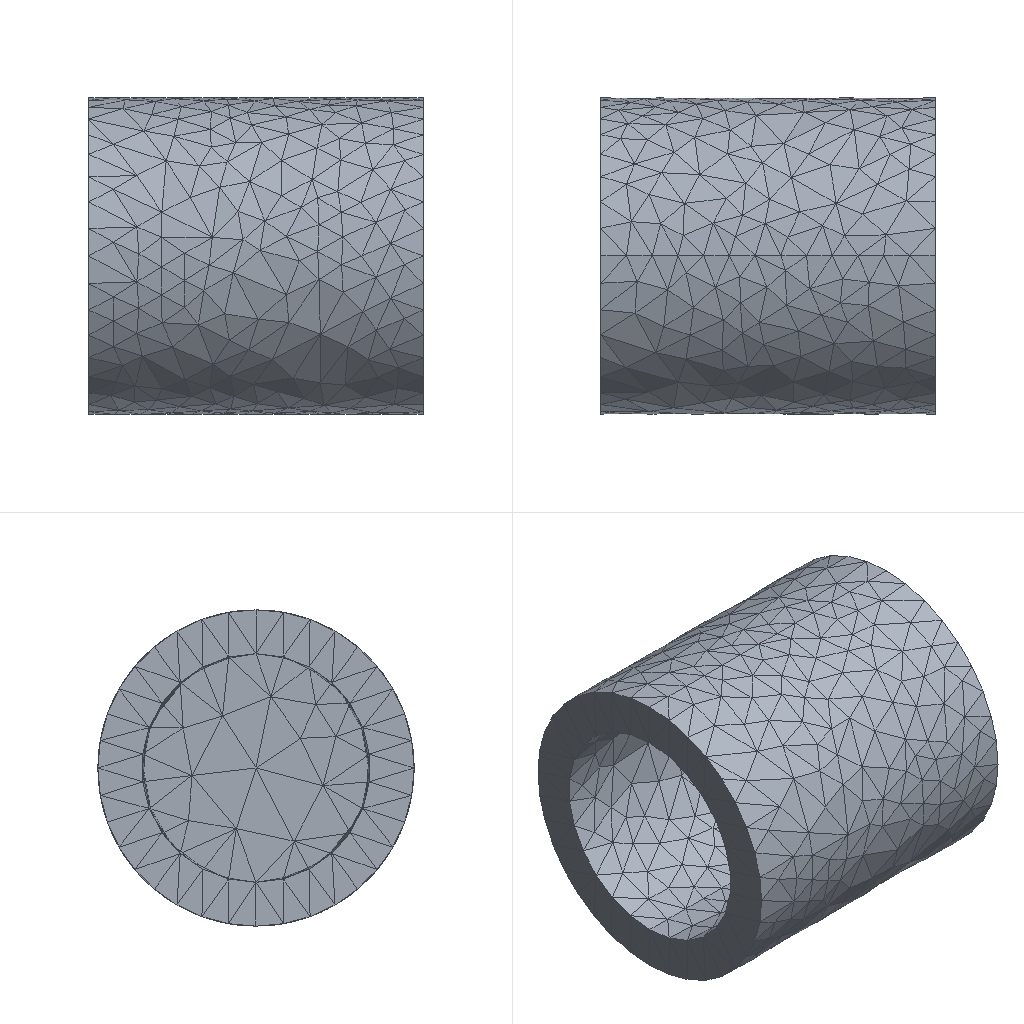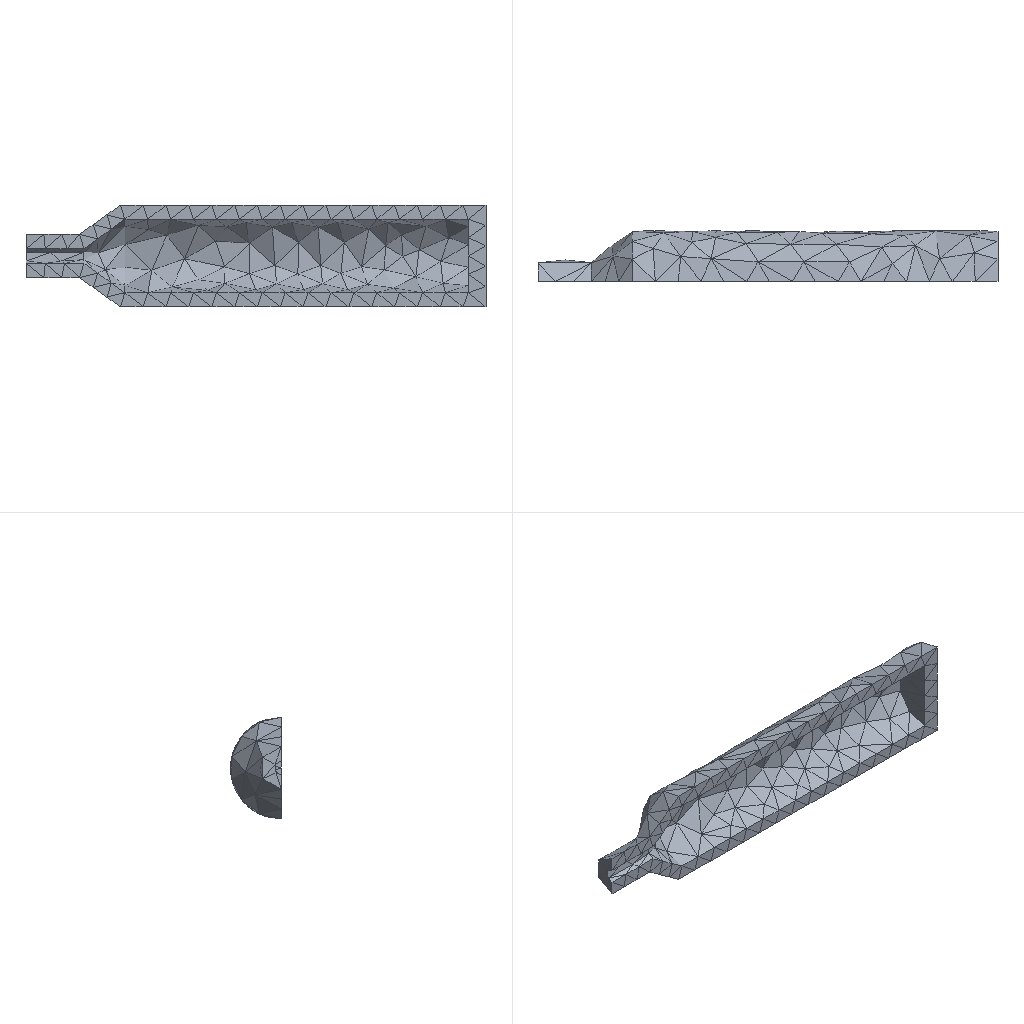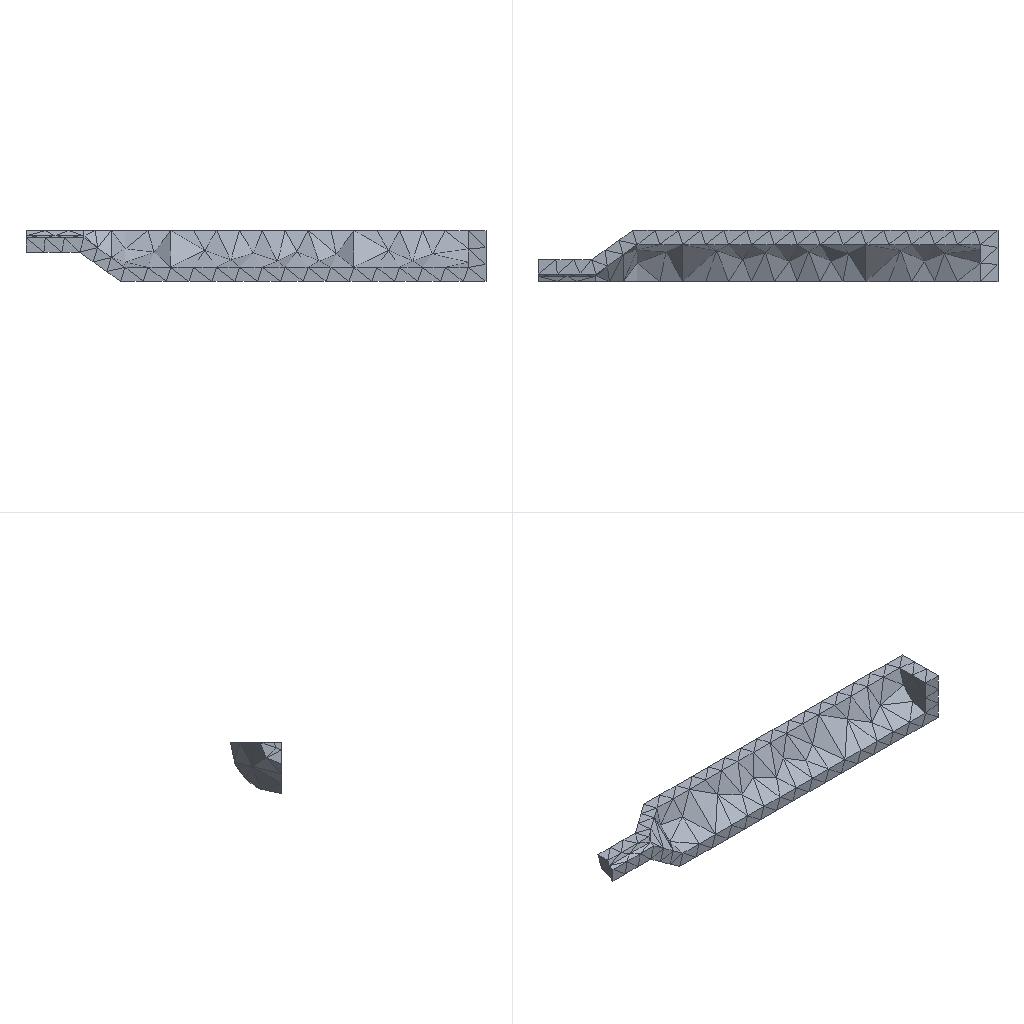Simulation study | ansys workbench
Set-up summary:
category,name,step,type,value,unit,region
solver,ansys_workbench
units,mm-N-s-tonne (MPa),,stated,"/units,MPA"
analysis,deck-1/LS1,,static
load_step,deck-1/LS1,deck-1/LS1,static,nsubst=1; time=1
analysis,deck-2/LS1,,static
load_step,deck-2/LS1,deck-2/LS1,static,nsubst=1; time=1
analysis,deck-3/LS1,,static
load_step,deck-3/LS1,deck-3/LS1,static,nsubst=1; time=1
mesh,deck-1.dat,,nodes,5359
mesh,deck-1.dat,,elements,4140
element_type,SOLID187,,,2968,,deck-1.dat
element_type,SURF154,,,1172,,deck-1.dat
mesh,deck-2.dat,,nodes,1306
mesh,deck-2.dat,,elements,880
element_type,SOLID187,,,578,,deck-2.dat
element_type,SURF154,,,302,,deck-2.dat
mesh,deck-3.dat,,nodes,759
mesh,deck-3.dat,,elements,453
element_type,SOLID187,,,303,,deck-3.dat
element_type,SURF154,,,150,,deck-3.dat
material,Structural Steel,,E,200000,tonne s^-2 mm^-1
material,Structural Steel,,nu,0.3
material,Structural Steel,,density,7.85e-09,tonne mm^-3
material,Structural Steel,,conductivity,60.5,tonne mm s^-3 C^-1
material,Structural Steel,,specific_heat,4.34e+08,mm^2 s^-2 C^-1
material,Structural Steel,,cte,1.2e-05,C^-1
material,Structural Steel,,permeability,10000
material,Structural Steel,,resistivity,0.00017,ohm mm
material,Structural Steel,,E,200000,tonne s^-2 mm^-1
material,Structural Steel,,nu,0.3
material,Structural Steel,,density,7.85e-09,tonne mm^-3
material,Structural Steel,,conductivity,60.5,tonne mm s^-3 C^-1
material,Structural Steel,,specific_heat,4.34e+08,mm^2 s^-2 C^-1
material,Structural Steel,,cte,1.2e-05,C^-1
material,Structural Steel,,permeability,10000
material,Structural Steel,,resistivity,0.00017,ohm mm
material,Structural Steel,,E,200000,tonne s^-2 mm^-1
material,Structural Steel,,nu,0.3
material,Structural Steel,,density,7.85e-09,tonne mm^-3
material,Structural Steel,,conductivity,60.5,tonne mm s^-3 C^-1
material,Structural Steel,,specific_heat,4.34e+08,mm^2 s^-2 C^-1
material,Structural Steel,,cte,1.2e-05,C^-1
material,Structural Steel,,permeability,10000
material,Structural Steel,,resistivity,0.00017,ohm mm
load,"Define Pressure Using Surface Effect Elements ""__""",deck-1/LS1,pressure,20,,SURF154 #2
load,"Define Pressure Using Surface Effect Elements ""__ 2""",deck-1/LS1,pressure,60,,SURF154 #3
load,"Define Pressure Using Surface Effect Elements ""__""",deck-2/LS1,pressure,60,,SURF154 #2
load,"Define Pressure Using Surface Effect Elements ""__ 2""",deck-2/LS1,pressure,20,,SURF154 #3
load,"Define Pressure Using Surface Effect Elements ""__""",deck-3/LS1,pressure,30,,SURF154 #2
load,"Define Pressure Using Surface Effect Elements ""__ 2""",deck-3/LS1,pressure,20,,SURF154 #3
bc,Fixed Supports,deck-1/model,fixed,[dofs=ALL],,_FIXEDSU
bc,Fixed Supports,deck-2/model,fixed,[dofs=ALL],,_FIXEDSU
bc,Fixed Supports,deck-3/model,fixed,[dofs=ALL],,_FIXEDSU
named_set,_FIXEDSU,,node,201
named_set,_FIXEDSU,,node,325
named_set,_FIXEDSU,,node,147
Results summary:
result,analyses[0].index,,,1
result,analyses[0].system,,,SYS
result,analyses[0].deck,,,deck-1.dat
result,analyses[0].solve_status,,,completed
result,analyses[0].analysis_type,,,static
result,analyses[0].physics,,,mechanical
result,analyses[0].unit_system,,,"NMM: mm, ton, N, s, mV, mA, degC"
result,analyses[0].n_sets,,,1
result,analyses[0].load_steps[0].set,set=1,,1
result,analyses[0].load_steps[0].time_or_freq,set=1,,1
result,analyses[0].load_steps[0].max_displacement_magnitude,set=1,,0.06823
result,analyses[0].load_steps[0].max_von_mises_nodal,set=1,,152.437
result,analyses[0].load_steps[0].reaction_force_sum_xyz[1],set=1,,8.0272e-09
result,analyses[0].load_steps[0].reaction_force_sum_xyz[2],set=1,,-1.33323e-08
result,analyses[0].load_steps[0].reaction_force_sum_xyz[3],set=1,,2.51015e-08
result,analyses[1].index,,,2
result,analyses[1].system,,,SYS-1
result,analyses[1].deck,,,deck-2.dat
result,analyses[1].solve_status,,,completed
result,analyses[1].analysis_type,,,static
result,analyses[1].physics,,,mechanical
result,analyses[1].unit_system,,,"NMM: mm, ton, N, s, mV, mA, degC"
result,analyses[1].n_sets,,,1
result,analyses[1].load_steps[0].set,set=1,,1
result,analyses[1].load_steps[0].time_or_freq,set=1,,1
result,analyses[1].load_steps[0].max_displacement_magnitude,set=1,,0.1087
result,analyses[1].load_steps[0].max_von_mises_nodal,set=1,,176.614
result,analyses[1].load_steps[0].reaction_force_sum_xyz[1],set=1,,-1.56621e-09
result,analyses[1].load_steps[0].reaction_force_sum_xyz[2],set=1,,-6.20424e+06
result,analyses[1].load_steps[0].reaction_force_sum_xyz[3],set=1,,-7.34008e-09
result,analyses[2].index,,,3
result,analyses[2].system,,,SYS-2
result,analyses[2].deck,,,deck-3.dat
result,analyses[2].solve_status,,,completed
result,analyses[2].analysis_type,,,static
result,analyses[2].physics,,,mechanical
result,analyses[2].unit_system,,,"NMM: mm, ton, N, s, mV, mA, degC"
result,analyses[2].n_sets,,,1
result,analyses[2].load_steps[0].set,set=1,,1
result,analyses[2].load_steps[0].time_or_freq,set=1,,1
result,analyses[2].load_steps[0].max_displacement_magnitude,set=1,,0.1895
result,analyses[2].load_steps[0].max_von_mises_nodal,set=1,,81.22
result,analyses[2].load_steps[0].reaction_force_sum_xyz[1],set=1,,-1.19874e-07
result,analyses[2].load_steps[0].reaction_force_sum_xyz[2],set=1,,-55368.1
result,analyses[2].load_steps[0].reaction_force_sum_xyz[3],set=1,,55368.1